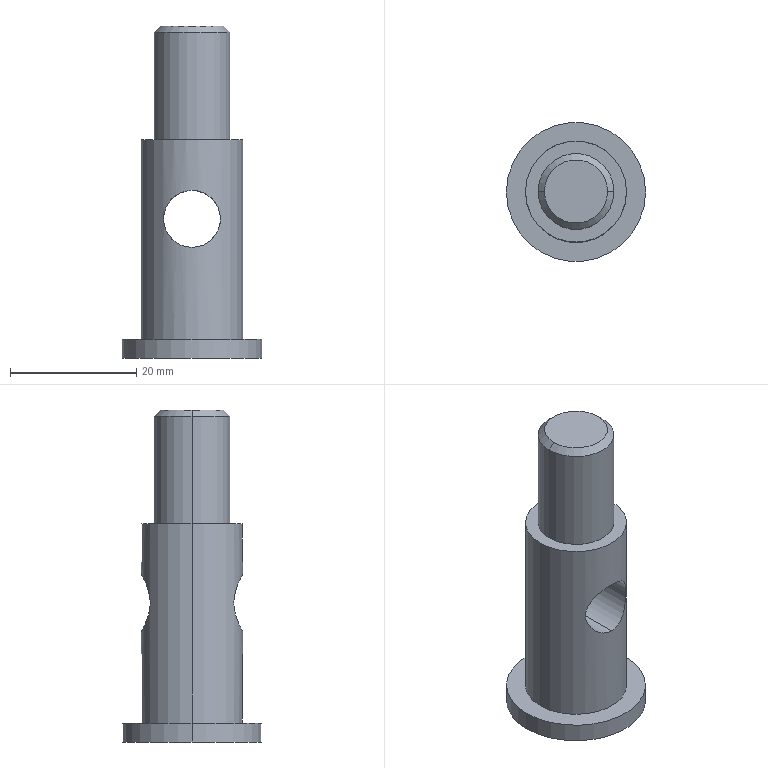Part | STEP file | Screen clamp adjusting rod 2 | 1 solid | 14 faces | box 22 x 22 x 52.5 mm | volume 8516 mm3 | cylinder 8 | plane 4 | cone 2 | commonest cylinder face diameters 9 x2 12 x2 16 x2 22 x2
STEP:
#1=CARTESIAN_POINT('',(5.,0.,52.5));
#2=VERTEX_POINT('',#1);
#3=CARTESIAN_POINT('',(-5.,0.,52.5));
#4=VERTEX_POINT('',#3);
#5=CARTESIAN_POINT('',(0.,0.,52.5));
#6=DIRECTION('',(0.,0.,1.));
#7=DIRECTION('',(1.,0.,0.));
#8=AXIS2_PLACEMENT_3D('',#5,#6,#7);
#9=CIRCLE('',#8,5.);
#10=EDGE_CURVE('',#2,#4,#9,.T.);
#11=ORIENTED_EDGE('',*,*,#10,.F.);
#12=CARTESIAN_POINT('',(6.,0.,51.5));
#13=VERTEX_POINT('',#12);
#14=CARTESIAN_POINT('',(5.,0.,52.5));
#15=DIRECTION('',(0.7071,0.,-0.7071));
#16=VECTOR('',#15,1000.);
#17=LINE('',#14,#16);
#18=EDGE_CURVE('',#2,#13,#17,.T.);
#19=ORIENTED_EDGE('',*,*,#18,.T.);
#20=CARTESIAN_POINT('',(-6.,0.,51.5));
#21=VERTEX_POINT('',#20);
#22=CARTESIAN_POINT('',(0.,0.,51.5));
#23=DIRECTION('',(0.,0.,-1.));
#24=DIRECTION('',(1.,0.,0.));
#25=AXIS2_PLACEMENT_3D('',#22,#23,#24);
#26=CIRCLE('',#25,6.);
#27=EDGE_CURVE('',#21,#13,#26,.T.);
#28=ORIENTED_EDGE('',*,*,#27,.F.);
#29=CARTESIAN_POINT('',(-5.,0.,52.5));
#30=DIRECTION('',(-0.7071,0.,-0.7071));
#31=VECTOR('',#30,1000.);
#32=LINE('',#29,#31);
#33=EDGE_CURVE('',#4,#21,#32,.T.);
#34=ORIENTED_EDGE('',*,*,#33,.F.);
#35=EDGE_LOOP('',(#11,#19,#28,#34));
#36=FACE_OUTER_BOUND('',#35,.T.);
#37=CARTESIAN_POINT('',(0.,0.,52.5));
#38=DIRECTION('',(0.,0.,-1.));
#39=DIRECTION('',(-1.,0.,0.));
#40=AXIS2_PLACEMENT_3D('',#37,#38,#39);
#41=CONICAL_SURFACE('',#40,5.,0.7854);
#42=ADVANCED_FACE('',(#36),#41,.T.);
#43=ORIENTED_EDGE('',*,*,#27,.T.);
#44=CARTESIAN_POINT('',(6.,0.,34.5));
#45=VERTEX_POINT('',#44);
#46=CARTESIAN_POINT('',(6.,0.,52.5));
#47=DIRECTION('',(0.,0.,-1.));
#48=VECTOR('',#47,1000.);
#49=LINE('',#46,#48);
#50=EDGE_CURVE('',#13,#45,#49,.T.);
#51=ORIENTED_EDGE('',*,*,#50,.T.);
#52=CARTESIAN_POINT('',(-6.,0.,34.5));
#53=VERTEX_POINT('',#52);
#54=CARTESIAN_POINT('',(0.,0.,34.5));
#55=DIRECTION('',(0.,0.,1.));
#56=DIRECTION('',(1.,0.,0.));
#57=AXIS2_PLACEMENT_3D('',#54,#55,#56);
#58=CIRCLE('',#57,6.);
#59=EDGE_CURVE('',#45,#53,#58,.T.);
#60=ORIENTED_EDGE('',*,*,#59,.T.);
#61=CARTESIAN_POINT('',(-6.,0.,52.5));
#62=DIRECTION('',(0.,0.,-1.));
#63=VECTOR('',#62,1000.);
#64=LINE('',#61,#63);
#65=EDGE_CURVE('',#21,#53,#64,.T.);
#66=ORIENTED_EDGE('',*,*,#65,.F.);
#67=EDGE_LOOP('',(#43,#51,#60,#66));
#68=FACE_OUTER_BOUND('',#67,.T.);
#69=CARTESIAN_POINT('',(0.,0.,52.5));
#70=DIRECTION('',(0.,0.,-1.));
#71=DIRECTION('',(-1.,0.,0.));
#72=AXIS2_PLACEMENT_3D('',#69,#70,#71);
#73=CYLINDRICAL_SURFACE('',#72,6.);
#74=ADVANCED_FACE('',(#68),#73,.T.);
#75=CARTESIAN_POINT('',(0.,-8.,17.5));
#76=VERTEX_POINT('',#75);
#77=CARTESIAN_POINT('',(0.,-8.,26.5));
#78=VERTEX_POINT('',#77);
#79=CARTESIAN_POINT('',(0.,-8.,17.5));
#80=CARTESIAN_POINT('',(-0.3039,-8.,17.5));
#81=CARTESIAN_POINT('',(-0.6032,-7.983,17.531));
#82=CARTESIAN_POINT('',(-1.188,-7.917,17.649));
#83=CARTESIAN_POINT('',(-1.477,-7.867,17.739));
#84=CARTESIAN_POINT('',(-2.021,-7.746,17.968));
#85=CARTESIAN_POINT('',(-2.277,-7.673,18.108));
#86=CARTESIAN_POINT('',(-2.762,-7.512,18.436));
#87=CARTESIAN_POINT('',(-2.985,-7.426,18.62));
#88=CARTESIAN_POINT('',(-3.39,-7.25,19.027));
#89=CARTESIAN_POINT('',(-3.575,-7.159,19.252));
#90=CARTESIAN_POINT('',(-3.897,-6.989,19.732));
#91=CARTESIAN_POINT('',(-4.035,-6.909,19.986));
#92=CARTESIAN_POINT('',(-4.261,-6.772,20.524));
#93=CARTESIAN_POINT('',(-4.351,-6.714,20.812));
#94=CARTESIAN_POINT('',(-4.469,-6.636,21.397));
#95=CARTESIAN_POINT('',(-4.5,-6.614,21.697));
#96=CARTESIAN_POINT('',(-4.5,-6.614,22.304));
#97=CARTESIAN_POINT('',(-4.469,-6.635,22.602));
#98=CARTESIAN_POINT('',(-4.351,-6.714,23.188));
#99=CARTESIAN_POINT('',(-4.261,-6.772,23.475));
#100=CARTESIAN_POINT('',(-4.034,-6.91,24.016));
#101=CARTESIAN_POINT('',(-3.894,-6.991,24.274));
#102=CARTESIAN_POINT('',(-3.57,-7.162,24.755));
#103=CARTESIAN_POINT('',(-3.387,-7.251,24.977));
#104=CARTESIAN_POINT('',(-2.98,-7.428,25.384));
#105=CARTESIAN_POINT('',(-2.754,-7.515,25.571));
#106=CARTESIAN_POINT('',(-2.274,-7.674,25.894));
#107=CARTESIAN_POINT('',(-2.018,-7.746,26.033));
#108=CARTESIAN_POINT('',(-1.61,-7.838,26.205));
#109=CARTESIAN_POINT('',(-1.468,-7.865,26.256));
#110=CARTESIAN_POINT('',(-1.184,-7.913,26.344));
#111=CARTESIAN_POINT('',(-1.04,-7.934,26.381));
#112=CARTESIAN_POINT('',(-0.6026,-7.983,26.469));
#113=CARTESIAN_POINT('',(-0.304,-8.,26.5));
#114=CARTESIAN_POINT('',(0.,-8.,26.5));
#115=B_SPLINE_CURVE_WITH_KNOTS('',3,(#79,#80,#81,#82,#83,#84,#85,#86,#87,#88,#89,#90,#91,#92,#93,#94,#95,#96,#97,#98,#99,#100,#101,#102,#103,#104,#105,#106,#107,#108,#109,#110,#111,#112,#113,#114),.UNSPECIFIED.,.F.,.F.,(4,2,2,2,2,2,2,2,2,2,2,2,2,2,2,2,2,4),(0.01439,0.01528,0.01618,0.01708,0.01798,0.01887,0.01977,0.02067,0.02157,0.02247,0.02336,0.02426,0.02516,0.02606,0.02695,0.0274,0.02785,0.02875),.UNSPECIFIED.);
#116=EDGE_CURVE('',#76,#78,#115,.T.);
#117=ORIENTED_EDGE('',*,*,#116,.F.);
#118=CARTESIAN_POINT('',(0.,8.,17.5));
#119=VERTEX_POINT('',#118);
#120=CARTESIAN_POINT('',(0.,10.,17.5));
#121=DIRECTION('',(0.,1.,0.));
#122=VECTOR('',#121,1000.);
#123=LINE('',#120,#122);
#124=EDGE_CURVE('',#76,#119,#123,.T.);
#125=ORIENTED_EDGE('',*,*,#124,.T.);
#126=CARTESIAN_POINT('',(0.,8.,26.5));
#127=VERTEX_POINT('',#126);
#128=CARTESIAN_POINT('',(0.,8.,26.5));
#129=CARTESIAN_POINT('',(-0.3044,8.,26.5));
#130=CARTESIAN_POINT('',(-0.6026,7.983,26.469));
#131=CARTESIAN_POINT('',(-1.187,7.917,26.351));
#132=CARTESIAN_POINT('',(-1.477,7.867,26.261));
#133=CARTESIAN_POINT('',(-2.02,7.746,26.032));
#134=CARTESIAN_POINT('',(-2.276,7.674,25.893));
#135=CARTESIAN_POINT('',(-2.761,7.513,25.566));
#136=CARTESIAN_POINT('',(-2.984,7.426,25.381));
#137=CARTESIAN_POINT('',(-3.389,7.25,24.974));
#138=CARTESIAN_POINT('',(-3.574,7.159,24.749));
#139=CARTESIAN_POINT('',(-3.897,6.989,24.269));
#140=CARTESIAN_POINT('',(-4.034,6.91,24.015));
#141=CARTESIAN_POINT('',(-4.261,6.772,23.477));
#142=CARTESIAN_POINT('',(-4.35,6.714,23.189));
#143=CARTESIAN_POINT('',(-4.469,6.636,22.604));
#144=CARTESIAN_POINT('',(-4.5,6.614,22.306));
#145=CARTESIAN_POINT('',(-4.5,6.614,21.697));
#146=CARTESIAN_POINT('',(-4.47,6.635,21.398));
#147=CARTESIAN_POINT('',(-4.351,6.714,20.813));
#148=CARTESIAN_POINT('',(-4.262,6.772,20.525));
#149=CARTESIAN_POINT('',(-4.034,6.91,19.985));
#150=CARTESIAN_POINT('',(-3.895,6.99,19.727));
#151=CARTESIAN_POINT('',(-3.57,7.162,19.245));
#152=CARTESIAN_POINT('',(-3.387,7.251,19.024));
#153=CARTESIAN_POINT('',(-2.981,7.427,18.616));
#154=CARTESIAN_POINT('',(-2.754,7.515,18.43));
#155=CARTESIAN_POINT('',(-2.274,7.674,18.106));
#156=CARTESIAN_POINT('',(-2.019,7.746,17.967));
#157=CARTESIAN_POINT('',(-1.611,7.837,17.796));
#158=CARTESIAN_POINT('',(-1.47,7.865,17.744));
#159=CARTESIAN_POINT('',(-1.184,7.913,17.656));
#160=CARTESIAN_POINT('',(-1.04,7.934,17.619));
#161=CARTESIAN_POINT('',(-0.6021,7.983,17.531));
#162=CARTESIAN_POINT('',(-0.3043,8.,17.5));
#163=CARTESIAN_POINT('',(0.,8.,17.5));
#164=B_SPLINE_CURVE_WITH_KNOTS('',3,(#128,#129,#130,#131,#132,#133,#134,#135,#136,#137,#138,#139,#140,#141,#142,#143,#144,#145,#146,#147,#148,#149,#150,#151,#152,#153,#154,#155,#156,#157,#158,#159,#160,#161,#162,#163),.UNSPECIFIED.,.F.,.F.,(4,2,2,2,2,2,2,2,2,2,2,2,2,2,2,2,2,4),(0.,0.0008991,0.001798,0.002697,0.003596,0.004496,0.005395,0.006294,0.007193,0.008092,0.008991,0.00989,0.01079,0.01169,0.01259,0.01304,0.01349,0.01439),.UNSPECIFIED.);
#165=EDGE_CURVE('',#127,#119,#164,.T.);
#166=ORIENTED_EDGE('',*,*,#165,.F.);
#167=CARTESIAN_POINT('',(0.,10.,26.5));
#168=DIRECTION('',(0.,1.,0.));
#169=VECTOR('',#168,1000.);
#170=LINE('',#167,#169);
#171=EDGE_CURVE('',#78,#127,#170,.T.);
#172=ORIENTED_EDGE('',*,*,#171,.F.);
#173=EDGE_LOOP('',(#117,#125,#166,#172));
#174=FACE_OUTER_BOUND('',#173,.T.);
#175=CARTESIAN_POINT('',(0.,10.,22.));
#176=DIRECTION('',(0.,1.,0.));
#177=DIRECTION('',(0.,0.,1.));
#178=AXIS2_PLACEMENT_3D('',#175,#176,#177);
#179=CYLINDRICAL_SURFACE('',#178,4.5);
#180=ADVANCED_FACE('',(#174),#179,.F.);
#181=ORIENTED_EDGE('',*,*,#165,.T.);
#182=CARTESIAN_POINT('',(0.,8.,17.5));
#183=CARTESIAN_POINT('',(0.3039,8.,17.5));
#184=CARTESIAN_POINT('',(0.6032,7.983,17.531));
#185=CARTESIAN_POINT('',(1.188,7.917,17.649));
#186=CARTESIAN_POINT('',(1.477,7.867,17.739));
#187=CARTESIAN_POINT('',(2.021,7.746,17.968));
#188=CARTESIAN_POINT('',(2.277,7.673,18.108));
#189=CARTESIAN_POINT('',(2.762,7.512,18.436));
#190=CARTESIAN_POINT('',(2.985,7.426,18.62));
#191=CARTESIAN_POINT('',(3.39,7.25,19.027));
#192=CARTESIAN_POINT('',(3.575,7.159,19.252));
#193=CARTESIAN_POINT('',(3.897,6.989,19.732));
#194=CARTESIAN_POINT('',(4.035,6.909,19.986));
#195=CARTESIAN_POINT('',(4.261,6.772,20.524));
#196=CARTESIAN_POINT('',(4.351,6.714,20.812));
#197=CARTESIAN_POINT('',(4.469,6.636,21.397));
#198=CARTESIAN_POINT('',(4.5,6.614,21.697));
#199=CARTESIAN_POINT('',(4.5,6.614,22.304));
#200=CARTESIAN_POINT('',(4.469,6.635,22.602));
#201=CARTESIAN_POINT('',(4.351,6.714,23.188));
#202=CARTESIAN_POINT('',(4.261,6.772,23.475));
#203=CARTESIAN_POINT('',(4.034,6.91,24.016));
#204=CARTESIAN_POINT('',(3.894,6.991,24.274));
#205=CARTESIAN_POINT('',(3.57,7.162,24.755));
#206=CARTESIAN_POINT('',(3.387,7.251,24.977));
#207=CARTESIAN_POINT('',(2.98,7.428,25.384));
#208=CARTESIAN_POINT('',(2.754,7.515,25.571));
#209=CARTESIAN_POINT('',(2.274,7.674,25.894));
#210=CARTESIAN_POINT('',(2.018,7.746,26.033));
#211=CARTESIAN_POINT('',(1.61,7.838,26.205));
#212=CARTESIAN_POINT('',(1.468,7.865,26.256));
#213=CARTESIAN_POINT('',(1.184,7.913,26.344));
#214=CARTESIAN_POINT('',(1.04,7.934,26.381));
#215=CARTESIAN_POINT('',(0.6026,7.983,26.469));
#216=CARTESIAN_POINT('',(0.304,8.,26.5));
#217=CARTESIAN_POINT('',(0.,8.,26.5));
#218=B_SPLINE_CURVE_WITH_KNOTS('',3,(#182,#183,#184,#185,#186,#187,#188,#189,#190,#191,#192,#193,#194,#195,#196,#197,#198,#199,#200,#201,#202,#203,#204,#205,#206,#207,#208,#209,#210,#211,#212,#213,#214,#215,#216,#217),.UNSPECIFIED.,.F.,.F.,(4,2,2,2,2,2,2,2,2,2,2,2,2,2,2,2,2,4),(0.01439,0.01528,0.01618,0.01708,0.01798,0.01887,0.01977,0.02067,0.02157,0.02247,0.02336,0.02426,0.02516,0.02606,0.02695,0.0274,0.02785,0.02875),.UNSPECIFIED.);
#219=EDGE_CURVE('',#119,#127,#218,.T.);
#220=ORIENTED_EDGE('',*,*,#219,.T.);
#221=EDGE_LOOP('',(#181,#220));
#222=FACE_BOUND('',#221,.T.);
#223=CARTESIAN_POINT('',(8.,0.,34.5));
#224=VERTEX_POINT('',#223);
#225=CARTESIAN_POINT('',(-8.,0.,34.5));
#226=VERTEX_POINT('',#225);
#227=CARTESIAN_POINT('',(0.,0.,34.5));
#228=DIRECTION('',(0.,0.,1.));
#229=DIRECTION('',(1.,0.,0.));
#230=AXIS2_PLACEMENT_3D('',#227,#228,#229);
#231=CIRCLE('',#230,8.);
#232=EDGE_CURVE('',#224,#226,#231,.T.);
#233=ORIENTED_EDGE('',*,*,#232,.F.);
#234=CARTESIAN_POINT('',(8.,0.,3.));
#235=VERTEX_POINT('',#234);
#236=CARTESIAN_POINT('',(8.,0.,34.5));
#237=DIRECTION('',(0.,0.,-1.));
#238=VECTOR('',#237,1000.);
#239=LINE('',#236,#238);
#240=EDGE_CURVE('',#224,#235,#239,.T.);
#241=ORIENTED_EDGE('',*,*,#240,.T.);
#242=CARTESIAN_POINT('',(-8.,0.,3.));
#243=VERTEX_POINT('',#242);
#244=CARTESIAN_POINT('',(0.,0.,3.));
#245=DIRECTION('',(0.,0.,1.));
#246=DIRECTION('',(1.,0.,0.));
#247=AXIS2_PLACEMENT_3D('',#244,#245,#246);
#248=CIRCLE('',#247,8.);
#249=EDGE_CURVE('',#235,#243,#248,.T.);
#250=ORIENTED_EDGE('',*,*,#249,.T.);
#251=CARTESIAN_POINT('',(-8.,0.,34.5));
#252=DIRECTION('',(0.,0.,-1.));
#253=VECTOR('',#252,1000.);
#254=LINE('',#251,#253);
#255=EDGE_CURVE('',#226,#243,#254,.T.);
#256=ORIENTED_EDGE('',*,*,#255,.F.);
#257=EDGE_LOOP('',(#233,#241,#250,#256));
#258=FACE_OUTER_BOUND('',#257,.T.);
#259=CARTESIAN_POINT('',(0.,0.,34.5));
#260=DIRECTION('',(0.,0.,-1.));
#261=DIRECTION('',(-1.,0.,0.));
#262=AXIS2_PLACEMENT_3D('',#259,#260,#261);
#263=CYLINDRICAL_SURFACE('',#262,8.);
#264=ADVANCED_FACE('',(#222,#258),#263,.T.);
#265=CARTESIAN_POINT('',(11.,0.,3.));
#266=VERTEX_POINT('',#265);
#267=CARTESIAN_POINT('',(-11.,0.,3.));
#268=VERTEX_POINT('',#267);
#269=CARTESIAN_POINT('',(0.,0.,3.));
#270=DIRECTION('',(0.,0.,1.));
#271=DIRECTION('',(1.,0.,0.));
#272=AXIS2_PLACEMENT_3D('',#269,#270,#271);
#273=CIRCLE('',#272,11.);
#274=EDGE_CURVE('',#266,#268,#273,.T.);
#275=ORIENTED_EDGE('',*,*,#274,.F.);
#276=CARTESIAN_POINT('',(11.,0.,0.));
#277=VERTEX_POINT('',#276);
#278=CARTESIAN_POINT('',(11.,0.,3.));
#279=DIRECTION('',(0.,0.,-1.));
#280=VECTOR('',#279,1000.);
#281=LINE('',#278,#280);
#282=EDGE_CURVE('',#266,#277,#281,.T.);
#283=ORIENTED_EDGE('',*,*,#282,.T.);
#284=CARTESIAN_POINT('',(-11.,0.,0.));
#285=VERTEX_POINT('',#284);
#286=CARTESIAN_POINT('',(0.,0.,0.));
#287=DIRECTION('',(0.,0.,1.));
#288=DIRECTION('',(1.,0.,0.));
#289=AXIS2_PLACEMENT_3D('',#286,#287,#288);
#290=CIRCLE('',#289,11.);
#291=EDGE_CURVE('',#277,#285,#290,.T.);
#292=ORIENTED_EDGE('',*,*,#291,.T.);
#293=CARTESIAN_POINT('',(-11.,0.,3.));
#294=DIRECTION('',(0.,0.,-1.));
#295=VECTOR('',#294,1000.);
#296=LINE('',#293,#295);
#297=EDGE_CURVE('',#268,#285,#296,.T.);
#298=ORIENTED_EDGE('',*,*,#297,.F.);
#299=EDGE_LOOP('',(#275,#283,#292,#298));
#300=FACE_OUTER_BOUND('',#299,.T.);
#301=CARTESIAN_POINT('',(0.,0.,3.));
#302=DIRECTION('',(0.,0.,-1.));
#303=DIRECTION('',(-1.,0.,0.));
#304=AXIS2_PLACEMENT_3D('',#301,#302,#303);
#305=CYLINDRICAL_SURFACE('',#304,11.);
#306=ADVANCED_FACE('',(#300),#305,.T.);
#307=CARTESIAN_POINT('',(0.,0.,34.5));
#308=DIRECTION('',(0.,0.,1.));
#309=DIRECTION('',(1.,0.,0.));
#310=AXIS2_PLACEMENT_3D('',#307,#308,#309);
#311=CIRCLE('',#310,8.);
#312=EDGE_CURVE('',#226,#224,#311,.T.);
#313=ORIENTED_EDGE('',*,*,#312,.T.);
#314=ORIENTED_EDGE('',*,*,#232,.T.);
#315=EDGE_LOOP('',(#313,#314));
#316=FACE_OUTER_BOUND('',#315,.T.);
#317=CARTESIAN_POINT('',(0.,0.,34.5));
#318=DIRECTION('',(0.,0.,1.));
#319=DIRECTION('',(1.,0.,0.));
#320=AXIS2_PLACEMENT_3D('',#317,#318,#319);
#321=CIRCLE('',#320,6.);
#322=EDGE_CURVE('',#53,#45,#321,.T.);
#323=ORIENTED_EDGE('',*,*,#322,.F.);
#324=ORIENTED_EDGE('',*,*,#59,.F.);
#325=EDGE_LOOP('',(#323,#324));
#326=FACE_BOUND('',#325,.T.);
#327=CARTESIAN_POINT('',(0.,0.,34.5));
#328=DIRECTION('',(0.,0.,1.));
#329=DIRECTION('',(1.,0.,0.));
#330=AXIS2_PLACEMENT_3D('',#327,#328,#329);
#331=PLANE('',#330);
#332=ADVANCED_FACE('',(#316,#326),#331,.T.);
#333=CARTESIAN_POINT('',(0.,0.,3.));
#334=DIRECTION('',(0.,0.,1.));
#335=DIRECTION('',(1.,0.,0.));
#336=AXIS2_PLACEMENT_3D('',#333,#334,#335);
#337=CIRCLE('',#336,11.);
#338=EDGE_CURVE('',#268,#266,#337,.T.);
#339=ORIENTED_EDGE('',*,*,#338,.T.);
#340=ORIENTED_EDGE('',*,*,#274,.T.);
#341=EDGE_LOOP('',(#339,#340));
#342=FACE_OUTER_BOUND('',#341,.T.);
#343=CARTESIAN_POINT('',(0.,0.,3.));
#344=DIRECTION('',(0.,0.,1.));
#345=DIRECTION('',(1.,0.,0.));
#346=AXIS2_PLACEMENT_3D('',#343,#344,#345);
#347=CIRCLE('',#346,8.);
#348=EDGE_CURVE('',#243,#235,#347,.T.);
#349=ORIENTED_EDGE('',*,*,#348,.F.);
#350=ORIENTED_EDGE('',*,*,#249,.F.);
#351=EDGE_LOOP('',(#349,#350));
#352=FACE_BOUND('',#351,.T.);
#353=CARTESIAN_POINT('',(0.,0.,3.));
#354=DIRECTION('',(0.,0.,1.));
#355=DIRECTION('',(1.,0.,0.));
#356=AXIS2_PLACEMENT_3D('',#353,#354,#355);
#357=PLANE('',#356);
#358=ADVANCED_FACE('',(#342,#352),#357,.T.);
#359=ORIENTED_EDGE('',*,*,#282,.F.);
#360=ORIENTED_EDGE('',*,*,#338,.F.);
#361=ORIENTED_EDGE('',*,*,#297,.T.);
#362=CARTESIAN_POINT('',(0.,0.,0.));
#363=DIRECTION('',(0.,0.,1.));
#364=DIRECTION('',(1.,0.,0.));
#365=AXIS2_PLACEMENT_3D('',#362,#363,#364);
#366=CIRCLE('',#365,11.);
#367=EDGE_CURVE('',#285,#277,#366,.T.);
#368=ORIENTED_EDGE('',*,*,#367,.T.);
#369=EDGE_LOOP('',(#359,#360,#361,#368));
#370=FACE_OUTER_BOUND('',#369,.T.);
#371=CARTESIAN_POINT('',(0.,0.,3.));
#372=DIRECTION('',(0.,0.,-1.));
#373=DIRECTION('',(-1.,0.,0.));
#374=AXIS2_PLACEMENT_3D('',#371,#372,#373);
#375=CYLINDRICAL_SURFACE('',#374,11.);
#376=ADVANCED_FACE('',(#370),#375,.T.);
#377=ORIENTED_EDGE('',*,*,#367,.F.);
#378=ORIENTED_EDGE('',*,*,#291,.F.);
#379=EDGE_LOOP('',(#377,#378));
#380=FACE_OUTER_BOUND('',#379,.T.);
#381=CARTESIAN_POINT('',(0.,0.,0.));
#382=DIRECTION('',(0.,0.,1.));
#383=DIRECTION('',(1.,0.,0.));
#384=AXIS2_PLACEMENT_3D('',#381,#382,#383);
#385=PLANE('',#384);
#386=ADVANCED_FACE('',(#380),#385,.F.);
#387=ORIENTED_EDGE('',*,*,#240,.F.);
#388=ORIENTED_EDGE('',*,*,#312,.F.);
#389=ORIENTED_EDGE('',*,*,#255,.T.);
#390=ORIENTED_EDGE('',*,*,#348,.T.);
#391=EDGE_LOOP('',(#387,#388,#389,#390));
#392=FACE_OUTER_BOUND('',#391,.T.);
#393=CARTESIAN_POINT('',(0.,-8.,26.5));
#394=CARTESIAN_POINT('',(0.3044,-8.,26.5));
#395=CARTESIAN_POINT('',(0.6026,-7.983,26.469));
#396=CARTESIAN_POINT('',(1.187,-7.917,26.351));
#397=CARTESIAN_POINT('',(1.477,-7.867,26.261));
#398=CARTESIAN_POINT('',(2.02,-7.746,26.032));
#399=CARTESIAN_POINT('',(2.276,-7.674,25.893));
#400=CARTESIAN_POINT('',(2.761,-7.513,25.566));
#401=CARTESIAN_POINT('',(2.984,-7.426,25.381));
#402=CARTESIAN_POINT('',(3.389,-7.25,24.974));
#403=CARTESIAN_POINT('',(3.574,-7.159,24.749));
#404=CARTESIAN_POINT('',(3.897,-6.989,24.269));
#405=CARTESIAN_POINT('',(4.034,-6.91,24.015));
#406=CARTESIAN_POINT('',(4.261,-6.772,23.477));
#407=CARTESIAN_POINT('',(4.35,-6.714,23.189));
#408=CARTESIAN_POINT('',(4.469,-6.636,22.604));
#409=CARTESIAN_POINT('',(4.5,-6.614,22.306));
#410=CARTESIAN_POINT('',(4.5,-6.614,21.697));
#411=CARTESIAN_POINT('',(4.47,-6.635,21.398));
#412=CARTESIAN_POINT('',(4.351,-6.714,20.813));
#413=CARTESIAN_POINT('',(4.262,-6.772,20.525));
#414=CARTESIAN_POINT('',(4.034,-6.91,19.985));
#415=CARTESIAN_POINT('',(3.895,-6.99,19.727));
#416=CARTESIAN_POINT('',(3.57,-7.162,19.245));
#417=CARTESIAN_POINT('',(3.387,-7.251,19.024));
#418=CARTESIAN_POINT('',(2.981,-7.427,18.616));
#419=CARTESIAN_POINT('',(2.754,-7.515,18.43));
#420=CARTESIAN_POINT('',(2.274,-7.674,18.106));
#421=CARTESIAN_POINT('',(2.019,-7.746,17.967));
#422=CARTESIAN_POINT('',(1.611,-7.837,17.796));
#423=CARTESIAN_POINT('',(1.47,-7.865,17.744));
#424=CARTESIAN_POINT('',(1.184,-7.913,17.656));
#425=CARTESIAN_POINT('',(1.04,-7.934,17.619));
#426=CARTESIAN_POINT('',(0.6021,-7.983,17.531));
#427=CARTESIAN_POINT('',(0.3043,-8.,17.5));
#428=CARTESIAN_POINT('',(0.,-8.,17.5));
#429=B_SPLINE_CURVE_WITH_KNOTS('',3,(#393,#394,#395,#396,#397,#398,#399,#400,#401,#402,#403,#404,#405,#406,#407,#408,#409,#410,#411,#412,#413,#414,#415,#416,#417,#418,#419,#420,#421,#422,#423,#424,#425,#426,#427,#428),.UNSPECIFIED.,.F.,.F.,(4,2,2,2,2,2,2,2,2,2,2,2,2,2,2,2,2,4),(0.,0.0008991,0.001798,0.002697,0.003596,0.004496,0.005395,0.006294,0.007193,0.008092,0.008991,0.00989,0.01079,0.01169,0.01259,0.01304,0.01349,0.01439),.UNSPECIFIED.);
#430=EDGE_CURVE('',#78,#76,#429,.T.);
#431=ORIENTED_EDGE('',*,*,#430,.T.);
#432=ORIENTED_EDGE('',*,*,#116,.T.);
#433=EDGE_LOOP('',(#431,#432));
#434=FACE_BOUND('',#433,.T.);
#435=CARTESIAN_POINT('',(0.,0.,34.5));
#436=DIRECTION('',(0.,0.,-1.));
#437=DIRECTION('',(-1.,0.,0.));
#438=AXIS2_PLACEMENT_3D('',#435,#436,#437);
#439=CYLINDRICAL_SURFACE('',#438,8.);
#440=ADVANCED_FACE('',(#392,#434),#439,.T.);
#441=ORIENTED_EDGE('',*,*,#124,.F.);
#442=ORIENTED_EDGE('',*,*,#430,.F.);
#443=ORIENTED_EDGE('',*,*,#171,.T.);
#444=ORIENTED_EDGE('',*,*,#219,.F.);
#445=EDGE_LOOP('',(#441,#442,#443,#444));
#446=FACE_OUTER_BOUND('',#445,.T.);
#447=CARTESIAN_POINT('',(0.,10.,22.));
#448=DIRECTION('',(0.,1.,0.));
#449=DIRECTION('',(0.,0.,1.));
#450=AXIS2_PLACEMENT_3D('',#447,#448,#449);
#451=CYLINDRICAL_SURFACE('',#450,4.5);
#452=ADVANCED_FACE('',(#446),#451,.F.);
#453=ORIENTED_EDGE('',*,*,#50,.F.);
#454=CARTESIAN_POINT('',(0.,0.,51.5));
#455=DIRECTION('',(0.,0.,-1.));
#456=DIRECTION('',(1.,0.,0.));
#457=AXIS2_PLACEMENT_3D('',#454,#455,#456);
#458=CIRCLE('',#457,6.);
#459=EDGE_CURVE('',#13,#21,#458,.T.);
#460=ORIENTED_EDGE('',*,*,#459,.T.);
#461=ORIENTED_EDGE('',*,*,#65,.T.);
#462=ORIENTED_EDGE('',*,*,#322,.T.);
#463=EDGE_LOOP('',(#453,#460,#461,#462));
#464=FACE_OUTER_BOUND('',#463,.T.);
#465=CARTESIAN_POINT('',(0.,0.,52.5));
#466=DIRECTION('',(0.,0.,-1.));
#467=DIRECTION('',(-1.,0.,0.));
#468=AXIS2_PLACEMENT_3D('',#465,#466,#467);
#469=CYLINDRICAL_SURFACE('',#468,6.);
#470=ADVANCED_FACE('',(#464),#469,.T.);
#471=CARTESIAN_POINT('',(0.,0.,52.5));
#472=DIRECTION('',(0.,0.,1.));
#473=DIRECTION('',(1.,0.,0.));
#474=AXIS2_PLACEMENT_3D('',#471,#472,#473);
#475=CIRCLE('',#474,5.);
#476=EDGE_CURVE('',#4,#2,#475,.T.);
#477=ORIENTED_EDGE('',*,*,#476,.T.);
#478=ORIENTED_EDGE('',*,*,#10,.T.);
#479=EDGE_LOOP('',(#477,#478));
#480=FACE_OUTER_BOUND('',#479,.T.);
#481=CARTESIAN_POINT('',(0.,0.,52.5));
#482=DIRECTION('',(0.,0.,1.));
#483=DIRECTION('',(1.,0.,0.));
#484=AXIS2_PLACEMENT_3D('',#481,#482,#483);
#485=PLANE('',#484);
#486=ADVANCED_FACE('',(#480),#485,.T.);
#487=ORIENTED_EDGE('',*,*,#18,.F.);
#488=ORIENTED_EDGE('',*,*,#476,.F.);
#489=ORIENTED_EDGE('',*,*,#33,.T.);
#490=ORIENTED_EDGE('',*,*,#459,.F.);
#491=EDGE_LOOP('',(#487,#488,#489,#490));
#492=FACE_OUTER_BOUND('',#491,.T.);
#493=CARTESIAN_POINT('',(0.,0.,52.5));
#494=DIRECTION('',(0.,0.,-1.));
#495=DIRECTION('',(-1.,0.,0.));
#496=AXIS2_PLACEMENT_3D('',#493,#494,#495);
#497=CONICAL_SURFACE('',#496,5.,0.7854);
#498=ADVANCED_FACE('',(#492),#497,.T.);
#499=CLOSED_SHELL('',(#42,#74,#180,#264,#306,#332,#358,#376,#386,#440,#452,#470,#486,#498));
#500=MANIFOLD_SOLID_BREP('',#499);
#501=CARTESIAN_POINT('',(0.,0.,0.));
#502=DIRECTION('',(0.,0.,1.));
#503=DIRECTION('',(1.,0.,0.));
#504=AXIS2_PLACEMENT_3D('',#501,#502,#503);
#505=(LENGTH_UNIT()NAMED_UNIT(*)SI_UNIT(.MILLI.,.METRE.));
#506=UNCERTAINTY_MEASURE_WITH_UNIT(LENGTH_MEASURE(0.00001),#505,'','');
#507=(NAMED_UNIT(*)PLANE_ANGLE_UNIT()SI_UNIT($,.RADIAN.));
#508=(NAMED_UNIT(*)SI_UNIT($,.STERADIAN.)SOLID_ANGLE_UNIT());
#509=(GEOMETRIC_REPRESENTATION_CONTEXT(3)GLOBAL_UNCERTAINTY_ASSIGNED_CONTEXT((#506))GLOBAL_UNIT_ASSIGNED_CONTEXT((#505,#507,#508))REPRESENTATION_CONTEXT('',''));
#510=ADVANCED_BREP_SHAPE_REPRESENTATION('',(#500,#504),#509);